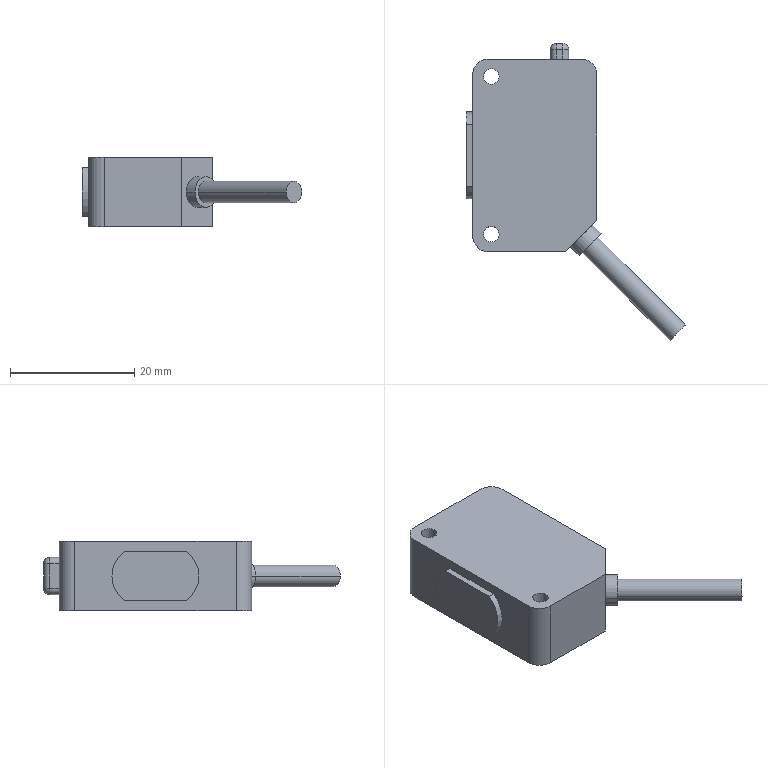Part | STEP file | Panasonic CX-444-P | 1 solid | 43 faces | box 35.294 x 47.794 x 11.2 mm | volume 7023 mm3 | cylinder 22 | plane 17 | sphere 4 | commonest cylinder face diameters 2 x8 5 x5 2.5 x4 10 x3 3.5 x2